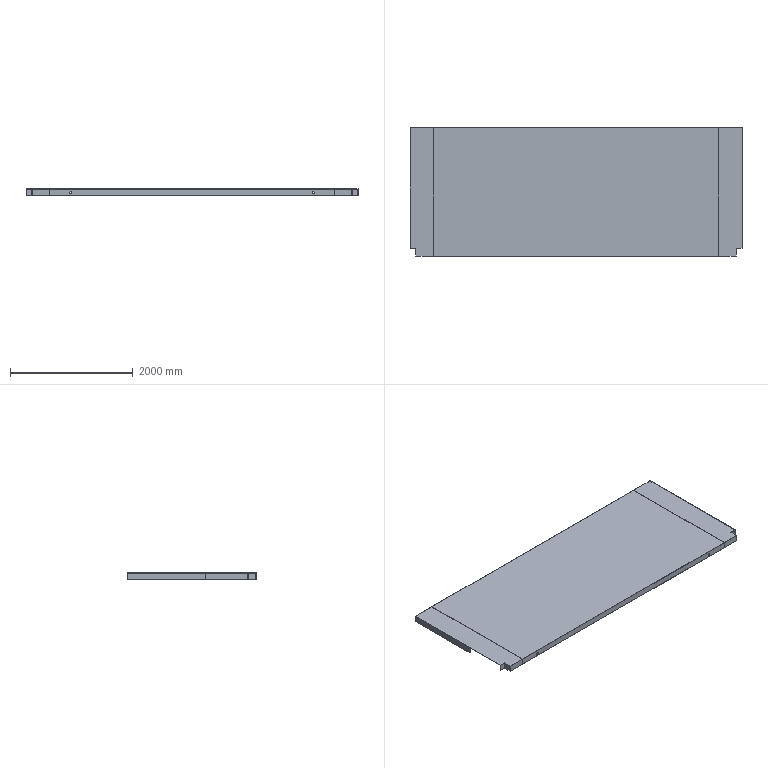Part | STEP file | PN_0041 second-floor passage platform plate_Default<As Machined> | 7 solids | 58 faces | box 5405 x 2088 x 103 mm | volume 36419067 mm3 | plane 56 | cylinder 2 | commonest cylinder face diameters 35 x2